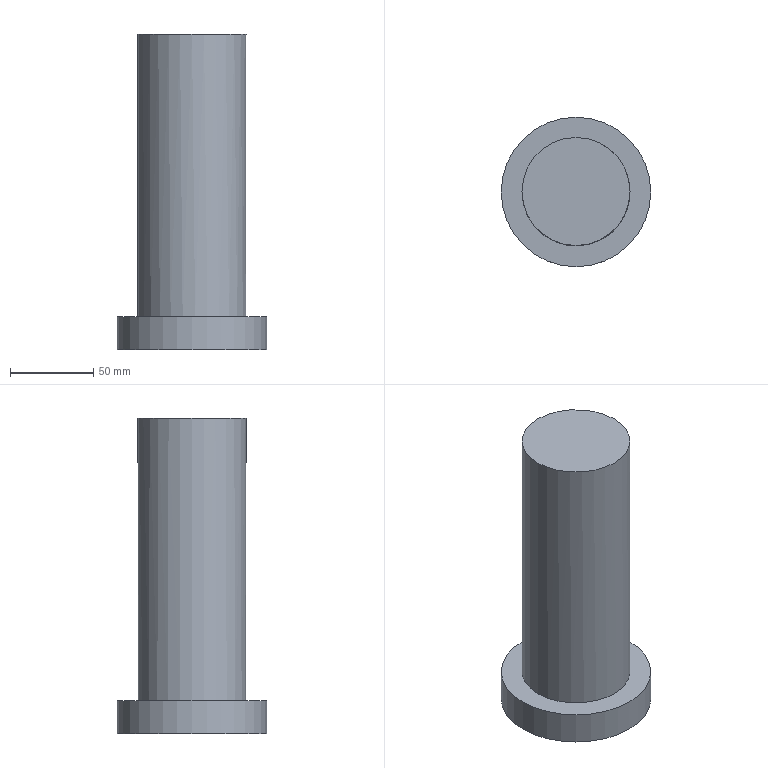Part | NX | features 平衡千斤顶活塞销 2 | 1 solid | 5 faces | box 90 x 90 x 190 mm | volume 691347 mm3 | plane 3 | cylinder 2 | commonest cylinder face diameters 65 x1 90 x1
STEP:
#1=CARTESIAN_POINT('',(32.5,0.,170.));
#2=VERTEX_POINT('',#1);
#3=CARTESIAN_POINT('',(0.,0.,170.));
#4=DIRECTION('',(0.,0.,1.));
#5=DIRECTION('',(1.,0.,0.));
#6=AXIS2_PLACEMENT_3D('',#3,#4,#5);
#7=CIRCLE('',#6,32.5);
#8=EDGE_CURVE('',#2,#2,#7,.T.);
#9=ORIENTED_EDGE('',*,*,#8,.F.);
#10=EDGE_LOOP('',(#9));
#11=FACE_BOUND('',#10,.T.);
#12=CARTESIAN_POINT('',(-32.5,0.,0.));
#13=VERTEX_POINT('',#12);
#14=CARTESIAN_POINT('',(0.,0.,0.));
#15=DIRECTION('',(0.,0.,-1.));
#16=DIRECTION('',(-1.,0.,0.));
#17=AXIS2_PLACEMENT_3D('',#14,#15,#16);
#18=CIRCLE('',#17,32.5);
#19=EDGE_CURVE('',#13,#13,#18,.T.);
#20=ORIENTED_EDGE('',*,*,#19,.F.);
#21=EDGE_LOOP('',(#20));
#22=FACE_BOUND('',#21,.T.);
#23=CARTESIAN_POINT('',(0.,0.,170.));
#24=DIRECTION('',(0.,0.,-1.));
#25=DIRECTION('',(-1.,0.,0.));
#26=AXIS2_PLACEMENT_3D('',#23,#24,#25);
#27=CYLINDRICAL_SURFACE('',#26,32.5);
#28=ADVANCED_FACE('',(#11,#22),#27,.T.);
#29=ORIENTED_EDGE('',*,*,#8,.T.);
#30=EDGE_LOOP('',(#29));
#31=FACE_BOUND('',#30,.T.);
#32=CARTESIAN_POINT('',(0.,0.,170.));
#33=DIRECTION('',(0.,0.,1.));
#34=DIRECTION('',(1.,0.,0.));
#35=AXIS2_PLACEMENT_3D('',#32,#33,#34);
#36=PLANE('',#35);
#37=ADVANCED_FACE('',(#31),#36,.T.);
#38=CARTESIAN_POINT('',(-45.,0.,0.));
#39=VERTEX_POINT('',#38);
#40=CARTESIAN_POINT('',(0.,0.,0.));
#41=DIRECTION('',(0.,0.,-1.));
#42=DIRECTION('',(-1.,0.,0.));
#43=AXIS2_PLACEMENT_3D('',#40,#41,#42);
#44=CIRCLE('',#43,45.);
#45=EDGE_CURVE('',#39,#39,#44,.T.);
#46=ORIENTED_EDGE('',*,*,#45,.F.);
#47=EDGE_LOOP('',(#46));
#48=FACE_BOUND('',#47,.T.);
#49=ORIENTED_EDGE('',*,*,#19,.T.);
#50=EDGE_LOOP('',(#49));
#51=FACE_BOUND('',#50,.T.);
#52=CARTESIAN_POINT('',(0.,0.,0.));
#53=DIRECTION('',(0.,0.,-1.));
#54=DIRECTION('',(-1.,0.,0.));
#55=AXIS2_PLACEMENT_3D('',#52,#53,#54);
#56=PLANE('',#55);
#57=ADVANCED_FACE('',(#48,#51),#56,.F.);
#58=CARTESIAN_POINT('',(-45.,0.,-20.));
#59=VERTEX_POINT('',#58);
#60=CARTESIAN_POINT('',(0.,0.,-20.));
#61=DIRECTION('',(0.,0.,-1.));
#62=DIRECTION('',(-1.,0.,0.));
#63=AXIS2_PLACEMENT_3D('',#60,#61,#62);
#64=CIRCLE('',#63,45.);
#65=EDGE_CURVE('',#59,#59,#64,.T.);
#66=ORIENTED_EDGE('',*,*,#65,.F.);
#67=EDGE_LOOP('',(#66));
#68=FACE_BOUND('',#67,.T.);
#69=ORIENTED_EDGE('',*,*,#45,.T.);
#70=EDGE_LOOP('',(#69));
#71=FACE_BOUND('',#70,.T.);
#72=CARTESIAN_POINT('',(0.,0.,-20.));
#73=DIRECTION('',(0.,0.,1.));
#74=DIRECTION('',(1.,0.,0.));
#75=AXIS2_PLACEMENT_3D('',#72,#73,#74);
#76=CYLINDRICAL_SURFACE('',#75,45.);
#77=ADVANCED_FACE('',(#68,#71),#76,.T.);
#78=ORIENTED_EDGE('',*,*,#65,.T.);
#79=EDGE_LOOP('',(#78));
#80=FACE_BOUND('',#79,.T.);
#81=CARTESIAN_POINT('',(0.,0.,-20.));
#82=DIRECTION('',(0.,0.,-1.));
#83=DIRECTION('',(-1.,0.,0.));
#84=AXIS2_PLACEMENT_3D('',#81,#82,#83);
#85=PLANE('',#84);
#86=ADVANCED_FACE('',(#80),#85,.T.);
#87=CLOSED_SHELL('',(#28,#37,#57,#77,#86));
#88=MANIFOLD_SOLID_BREP('',#87);
#89=(LENGTH_UNIT()NAMED_UNIT(*)SI_UNIT(.MILLI.,.METRE.));
#90=UNCERTAINTY_MEASURE_WITH_UNIT(LENGTH_MEASURE(0.00001),#89,'','');
#91=(NAMED_UNIT(*)PLANE_ANGLE_UNIT()SI_UNIT($,.RADIAN.));
#92=(NAMED_UNIT(*)SI_UNIT($,.STERADIAN.)SOLID_ANGLE_UNIT());
#93=(GEOMETRIC_REPRESENTATION_CONTEXT(3)GLOBAL_UNCERTAINTY_ASSIGNED_CONTEXT((#90))GLOBAL_UNIT_ASSIGNED_CONTEXT((#89,#91,#92))REPRESENTATION_CONTEXT('',''));
#94=ADVANCED_BREP_SHAPE_REPRESENTATION('',(#88),#93);